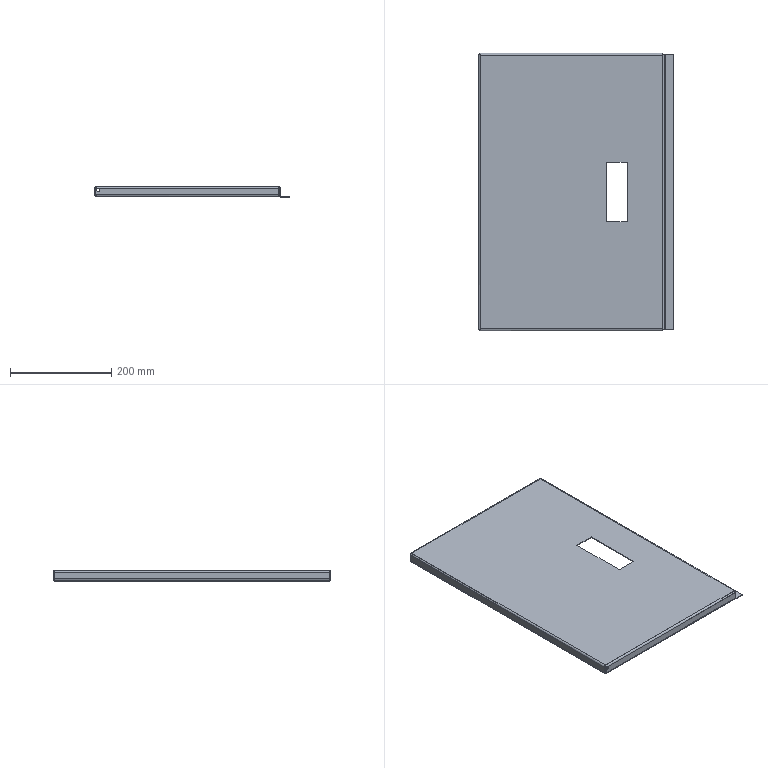Part | SolidWorks | features EdgeFlange 3, ICE 2, Fillet 1, FlatPattern 1, SMBaseFlange 1, SheetMetal 1 | 1 solid | 80 faces | box 384.5 x 547 x 21.5 mm | volume 378210 mm3 | plane 46 | cylinder 22 | spline 12 | commonest cylinder face diameters 4 x10 7 x8 6 x4